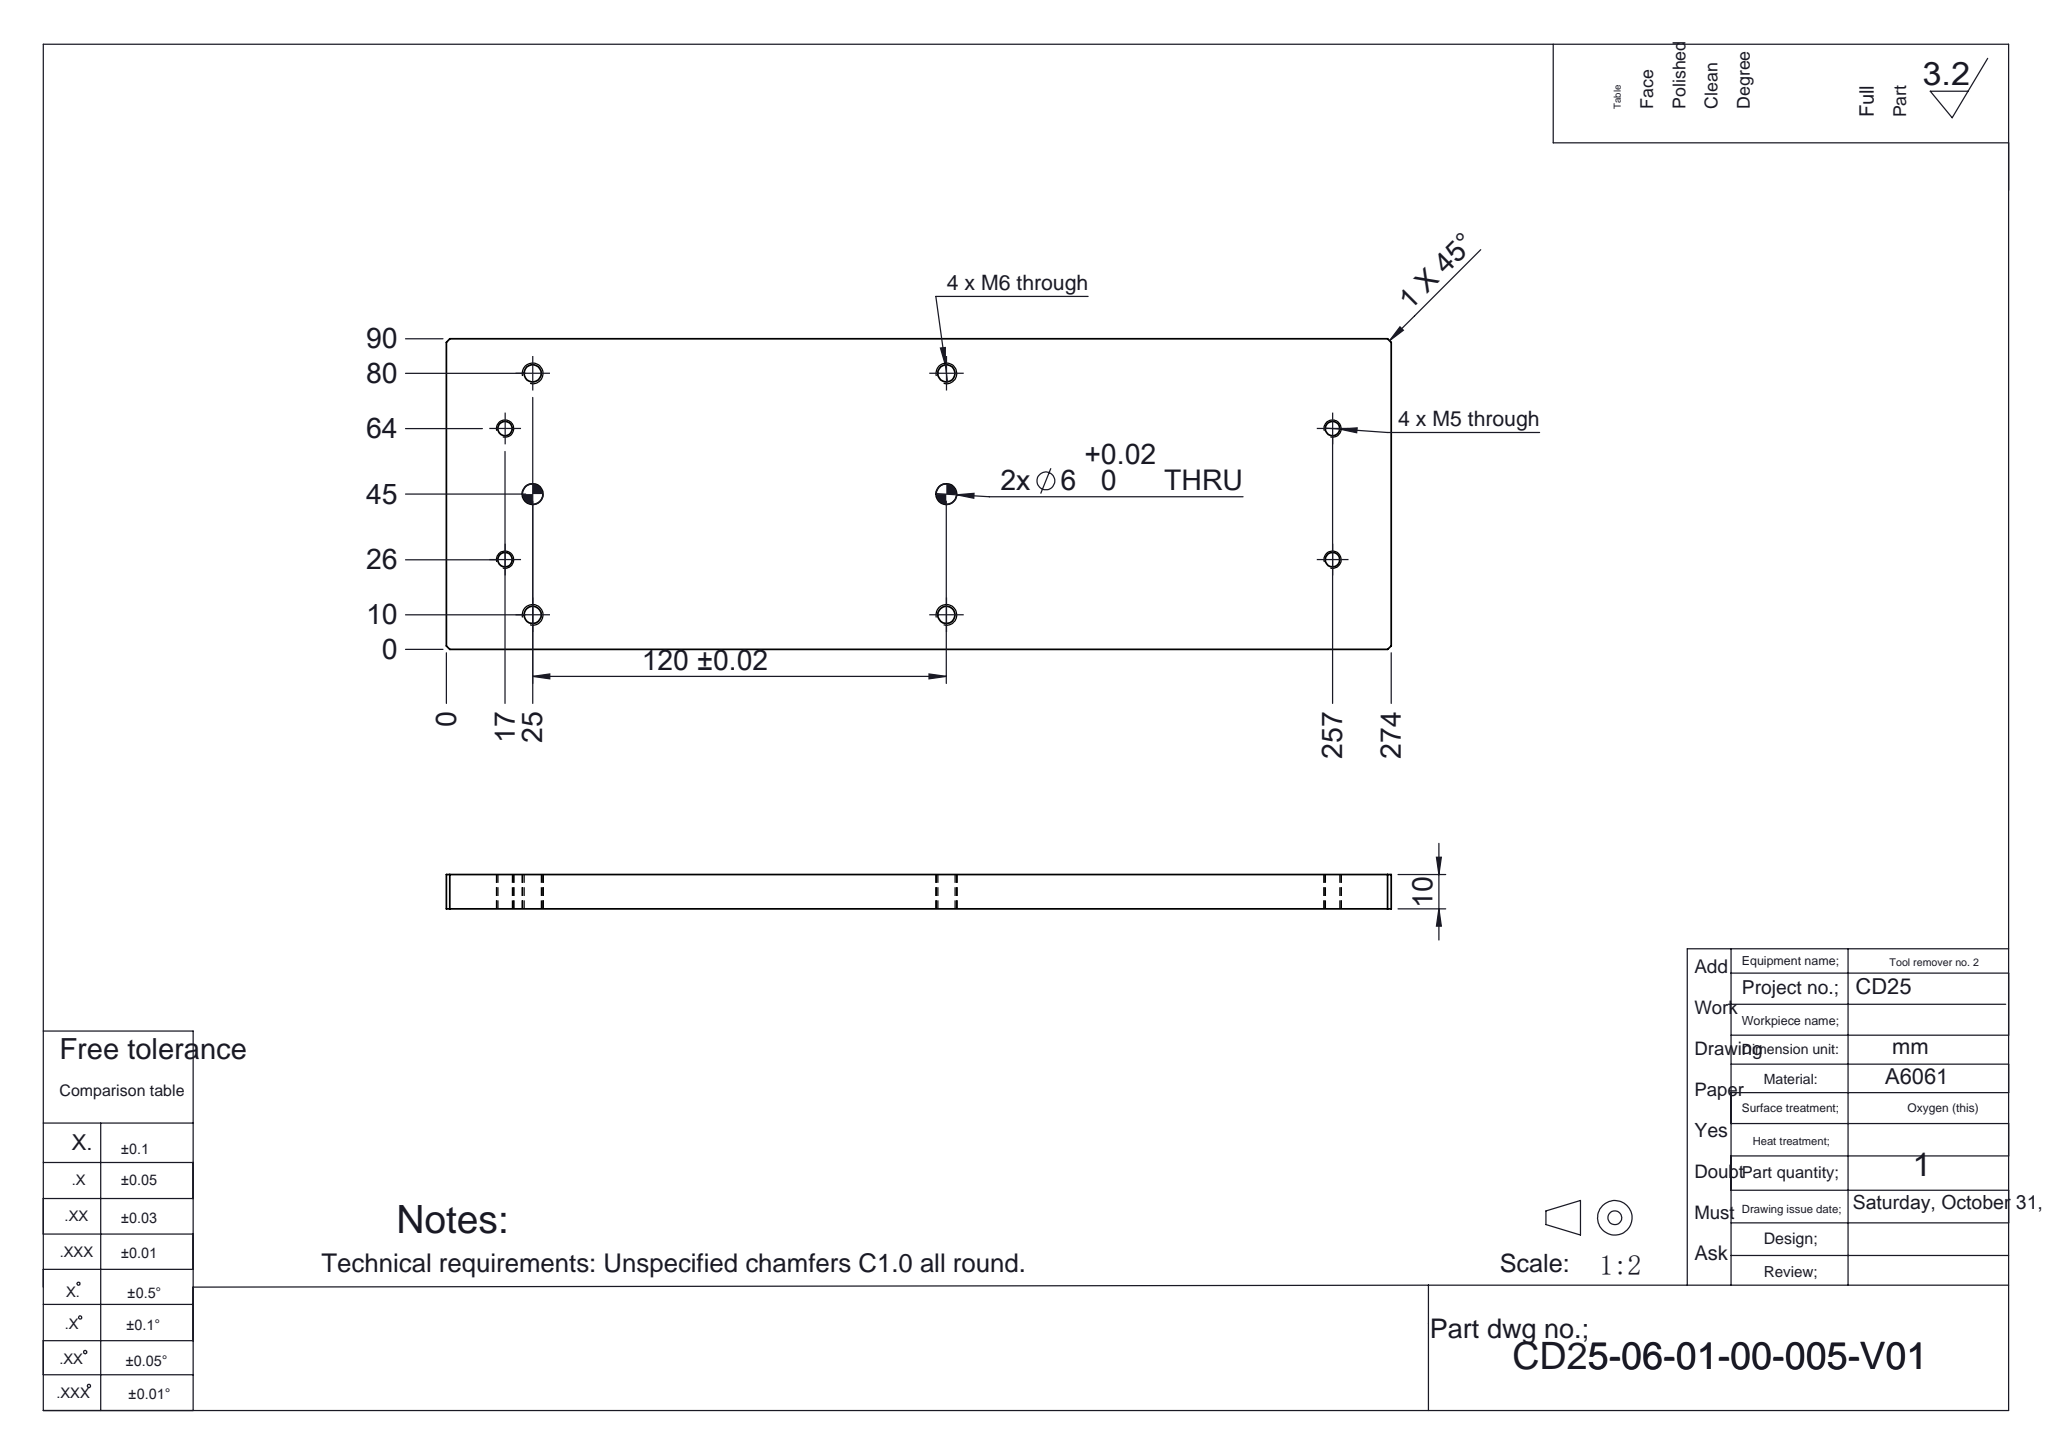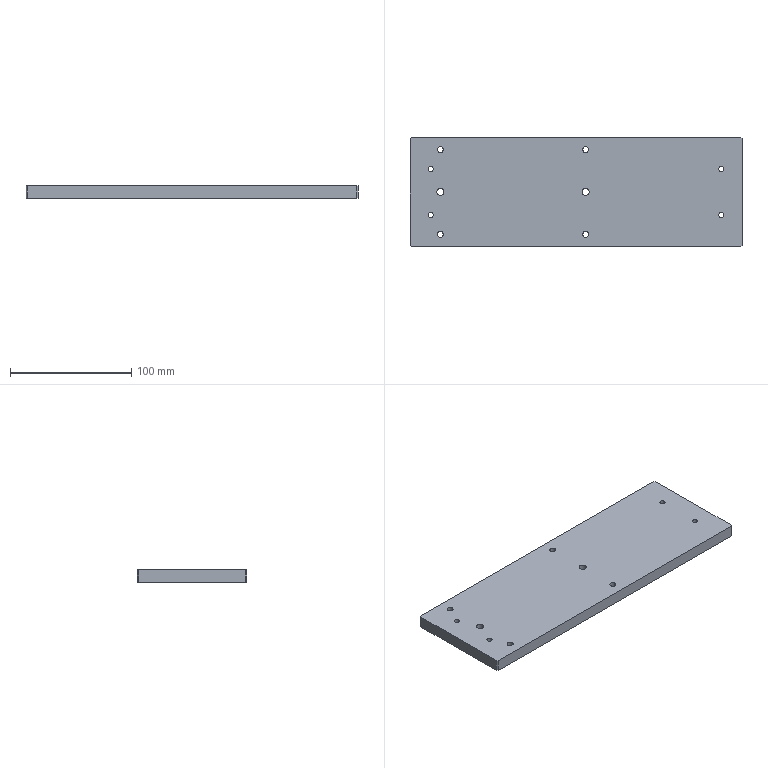Part | SolidWorks | features HoleWzd 3, Chamfer 1, Extrusion 1 | 1 solid | 30 faces | box 274 x 90 x 10 mm | volume 244675 mm3 | cylinder 20 | plane 10 | commonest cylinder face diameters 4.2 x8 5 x8 6 x4
STEP:
#1=CARTESIAN_POINT('',(-109.,0.,5.));
#2=VERTEX_POINT('',#1);
#3=CARTESIAN_POINT('',(-115.,0.,5.));
#4=VERTEX_POINT('',#3);
#5=CARTESIAN_POINT('',(-112.,0.,5.));
#6=DIRECTION('',(0.,0.,-1.));
#7=DIRECTION('',(-1.,0.,0.));
#8=AXIS2_PLACEMENT_3D('',#5,#6,#7);
#9=CIRCLE('',#8,3.);
#10=EDGE_CURVE('',#2,#4,#9,.T.);
#11=ORIENTED_EDGE('',*,*,#10,.F.);
#12=CARTESIAN_POINT('',(-109.,0.,-5.));
#13=VERTEX_POINT('',#12);
#14=CARTESIAN_POINT('',(-109.,0.,-5.));
#15=DIRECTION('',(0.,0.,-1.));
#16=VECTOR('',#15,1000.);
#17=LINE('',#14,#16);
#18=EDGE_CURVE('',#2,#13,#17,.T.);
#19=ORIENTED_EDGE('',*,*,#18,.T.);
#20=CARTESIAN_POINT('',(-115.,0.,-5.));
#21=VERTEX_POINT('',#20);
#22=CARTESIAN_POINT('',(-112.,0.,-5.));
#23=DIRECTION('',(0.,0.,-1.));
#24=DIRECTION('',(-1.,0.,0.));
#25=AXIS2_PLACEMENT_3D('',#22,#23,#24);
#26=CIRCLE('',#25,3.);
#27=EDGE_CURVE('',#13,#21,#26,.T.);
#28=ORIENTED_EDGE('',*,*,#27,.T.);
#29=CARTESIAN_POINT('',(-115.,0.,-5.));
#30=DIRECTION('',(0.,0.,-1.));
#31=VECTOR('',#30,1000.);
#32=LINE('',#29,#31);
#33=EDGE_CURVE('',#4,#21,#32,.T.);
#34=ORIENTED_EDGE('',*,*,#33,.F.);
#35=EDGE_LOOP('',(#11,#19,#28,#34));
#36=FACE_OUTER_BOUND('',#35,.T.);
#37=CARTESIAN_POINT('',(-112.,0.,-5.));
#38=DIRECTION('',(0.,0.,-1.));
#39=DIRECTION('',(-1.,0.,0.));
#40=AXIS2_PLACEMENT_3D('',#37,#38,#39);
#41=CYLINDRICAL_SURFACE('',#40,3.);
#42=ADVANCED_FACE('',(#36),#41,.F.);
#43=CARTESIAN_POINT('',(11.,0.,5.));
#44=VERTEX_POINT('',#43);
#45=CARTESIAN_POINT('',(5.,0.,5.));
#46=VERTEX_POINT('',#45);
#47=CARTESIAN_POINT('',(8.,0.,5.));
#48=DIRECTION('',(0.,0.,-1.));
#49=DIRECTION('',(-1.,0.,0.));
#50=AXIS2_PLACEMENT_3D('',#47,#48,#49);
#51=CIRCLE('',#50,3.);
#52=EDGE_CURVE('',#44,#46,#51,.T.);
#53=ORIENTED_EDGE('',*,*,#52,.F.);
#54=CARTESIAN_POINT('',(11.,0.,-5.));
#55=VERTEX_POINT('',#54);
#56=CARTESIAN_POINT('',(11.,0.,-5.));
#57=DIRECTION('',(0.,0.,-1.));
#58=VECTOR('',#57,1000.);
#59=LINE('',#56,#58);
#60=EDGE_CURVE('',#44,#55,#59,.T.);
#61=ORIENTED_EDGE('',*,*,#60,.T.);
#62=CARTESIAN_POINT('',(5.,0.,-5.));
#63=VERTEX_POINT('',#62);
#64=CARTESIAN_POINT('',(8.,0.,-5.));
#65=DIRECTION('',(0.,0.,-1.));
#66=DIRECTION('',(-1.,0.,0.));
#67=AXIS2_PLACEMENT_3D('',#64,#65,#66);
#68=CIRCLE('',#67,3.);
#69=EDGE_CURVE('',#55,#63,#68,.T.);
#70=ORIENTED_EDGE('',*,*,#69,.T.);
#71=CARTESIAN_POINT('',(5.,0.,-5.));
#72=DIRECTION('',(0.,0.,-1.));
#73=VECTOR('',#72,1000.);
#74=LINE('',#71,#73);
#75=EDGE_CURVE('',#46,#63,#74,.T.);
#76=ORIENTED_EDGE('',*,*,#75,.F.);
#77=EDGE_LOOP('',(#53,#61,#70,#76));
#78=FACE_OUTER_BOUND('',#77,.T.);
#79=CARTESIAN_POINT('',(8.,0.,-5.));
#80=DIRECTION('',(0.,0.,-1.));
#81=DIRECTION('',(-1.,0.,0.));
#82=AXIS2_PLACEMENT_3D('',#79,#80,#81);
#83=CYLINDRICAL_SURFACE('',#82,3.);
#84=ADVANCED_FACE('',(#78),#83,.F.);
#85=CARTESIAN_POINT('',(-109.5,35.,5.));
#86=VERTEX_POINT('',#85);
#87=CARTESIAN_POINT('',(-114.5,35.,5.));
#88=VERTEX_POINT('',#87);
#89=CARTESIAN_POINT('',(-112.,35.,5.));
#90=DIRECTION('',(0.,0.,-1.));
#91=DIRECTION('',(-1.,0.,0.));
#92=AXIS2_PLACEMENT_3D('',#89,#90,#91);
#93=CIRCLE('',#92,2.5);
#94=EDGE_CURVE('',#86,#88,#93,.T.);
#95=ORIENTED_EDGE('',*,*,#94,.F.);
#96=CARTESIAN_POINT('',(-109.5,35.,-5.));
#97=VERTEX_POINT('',#96);
#98=CARTESIAN_POINT('',(-109.5,35.,-5.));
#99=DIRECTION('',(0.,0.,-1.));
#100=VECTOR('',#99,1000.);
#101=LINE('',#98,#100);
#102=EDGE_CURVE('',#86,#97,#101,.T.);
#103=ORIENTED_EDGE('',*,*,#102,.T.);
#104=CARTESIAN_POINT('',(-114.5,35.,-5.));
#105=VERTEX_POINT('',#104);
#106=CARTESIAN_POINT('',(-112.,35.,-5.));
#107=DIRECTION('',(0.,0.,-1.));
#108=DIRECTION('',(-1.,0.,0.));
#109=AXIS2_PLACEMENT_3D('',#106,#107,#108);
#110=CIRCLE('',#109,2.5);
#111=EDGE_CURVE('',#97,#105,#110,.T.);
#112=ORIENTED_EDGE('',*,*,#111,.T.);
#113=CARTESIAN_POINT('',(-114.5,35.,-5.));
#114=DIRECTION('',(0.,0.,-1.));
#115=VECTOR('',#114,1000.);
#116=LINE('',#113,#115);
#117=EDGE_CURVE('',#88,#105,#116,.T.);
#118=ORIENTED_EDGE('',*,*,#117,.F.);
#119=EDGE_LOOP('',(#95,#103,#112,#118));
#120=FACE_OUTER_BOUND('',#119,.T.);
#121=CARTESIAN_POINT('',(-112.,35.,-5.));
#122=DIRECTION('',(0.,0.,-1.));
#123=DIRECTION('',(-1.,0.,0.));
#124=AXIS2_PLACEMENT_3D('',#121,#122,#123);
#125=CYLINDRICAL_SURFACE('',#124,2.5);
#126=ADVANCED_FACE('',(#120),#125,.F.);
#127=CARTESIAN_POINT('',(-109.5,-35.,5.));
#128=VERTEX_POINT('',#127);
#129=CARTESIAN_POINT('',(-114.5,-35.,5.));
#130=VERTEX_POINT('',#129);
#131=CARTESIAN_POINT('',(-112.,-35.,5.));
#132=DIRECTION('',(0.,0.,-1.));
#133=DIRECTION('',(-1.,0.,0.));
#134=AXIS2_PLACEMENT_3D('',#131,#132,#133);
#135=CIRCLE('',#134,2.5);
#136=EDGE_CURVE('',#128,#130,#135,.T.);
#137=ORIENTED_EDGE('',*,*,#136,.F.);
#138=CARTESIAN_POINT('',(-109.5,-35.,-5.));
#139=VERTEX_POINT('',#138);
#140=CARTESIAN_POINT('',(-109.5,-35.,-5.));
#141=DIRECTION('',(0.,0.,-1.));
#142=VECTOR('',#141,1000.);
#143=LINE('',#140,#142);
#144=EDGE_CURVE('',#128,#139,#143,.T.);
#145=ORIENTED_EDGE('',*,*,#144,.T.);
#146=CARTESIAN_POINT('',(-114.5,-35.,-5.));
#147=VERTEX_POINT('',#146);
#148=CARTESIAN_POINT('',(-112.,-35.,-5.));
#149=DIRECTION('',(0.,0.,-1.));
#150=DIRECTION('',(-1.,0.,0.));
#151=AXIS2_PLACEMENT_3D('',#148,#149,#150);
#152=CIRCLE('',#151,2.5);
#153=EDGE_CURVE('',#139,#147,#152,.T.);
#154=ORIENTED_EDGE('',*,*,#153,.T.);
#155=CARTESIAN_POINT('',(-114.5,-35.,-5.));
#156=DIRECTION('',(0.,0.,-1.));
#157=VECTOR('',#156,1000.);
#158=LINE('',#155,#157);
#159=EDGE_CURVE('',#130,#147,#158,.T.);
#160=ORIENTED_EDGE('',*,*,#159,.F.);
#161=EDGE_LOOP('',(#137,#145,#154,#160));
#162=FACE_OUTER_BOUND('',#161,.T.);
#163=CARTESIAN_POINT('',(-112.,-35.,-5.));
#164=DIRECTION('',(0.,0.,-1.));
#165=DIRECTION('',(-1.,0.,0.));
#166=AXIS2_PLACEMENT_3D('',#163,#164,#165);
#167=CYLINDRICAL_SURFACE('',#166,2.5);
#168=ADVANCED_FACE('',(#162),#167,.F.);
#169=CARTESIAN_POINT('',(10.5,-35.,5.));
#170=VERTEX_POINT('',#169);
#171=CARTESIAN_POINT('',(5.5,-35.,5.));
#172=VERTEX_POINT('',#171);
#173=CARTESIAN_POINT('',(8.,-35.,5.));
#174=DIRECTION('',(0.,0.,-1.));
#175=DIRECTION('',(-1.,0.,0.));
#176=AXIS2_PLACEMENT_3D('',#173,#174,#175);
#177=CIRCLE('',#176,2.5);
#178=EDGE_CURVE('',#170,#172,#177,.T.);
#179=ORIENTED_EDGE('',*,*,#178,.F.);
#180=CARTESIAN_POINT('',(10.5,-35.,-5.));
#181=VERTEX_POINT('',#180);
#182=CARTESIAN_POINT('',(10.5,-35.,-5.));
#183=DIRECTION('',(0.,0.,-1.));
#184=VECTOR('',#183,1000.);
#185=LINE('',#182,#184);
#186=EDGE_CURVE('',#170,#181,#185,.T.);
#187=ORIENTED_EDGE('',*,*,#186,.T.);
#188=CARTESIAN_POINT('',(5.5,-35.,-5.));
#189=VERTEX_POINT('',#188);
#190=CARTESIAN_POINT('',(8.,-35.,-5.));
#191=DIRECTION('',(0.,0.,-1.));
#192=DIRECTION('',(-1.,0.,0.));
#193=AXIS2_PLACEMENT_3D('',#190,#191,#192);
#194=CIRCLE('',#193,2.5);
#195=EDGE_CURVE('',#181,#189,#194,.T.);
#196=ORIENTED_EDGE('',*,*,#195,.T.);
#197=CARTESIAN_POINT('',(5.5,-35.,-5.));
#198=DIRECTION('',(0.,0.,-1.));
#199=VECTOR('',#198,1000.);
#200=LINE('',#197,#199);
#201=EDGE_CURVE('',#172,#189,#200,.T.);
#202=ORIENTED_EDGE('',*,*,#201,.F.);
#203=EDGE_LOOP('',(#179,#187,#196,#202));
#204=FACE_OUTER_BOUND('',#203,.T.);
#205=CARTESIAN_POINT('',(8.,-35.,-5.));
#206=DIRECTION('',(0.,0.,-1.));
#207=DIRECTION('',(-1.,0.,0.));
#208=AXIS2_PLACEMENT_3D('',#205,#206,#207);
#209=CYLINDRICAL_SURFACE('',#208,2.5);
#210=ADVANCED_FACE('',(#204),#209,.F.);
#211=CARTESIAN_POINT('',(10.5,35.,5.));
#212=VERTEX_POINT('',#211);
#213=CARTESIAN_POINT('',(5.5,35.,5.));
#214=VERTEX_POINT('',#213);
#215=CARTESIAN_POINT('',(8.,35.,5.));
#216=DIRECTION('',(0.,0.,-1.));
#217=DIRECTION('',(-1.,0.,0.));
#218=AXIS2_PLACEMENT_3D('',#215,#216,#217);
#219=CIRCLE('',#218,2.5);
#220=EDGE_CURVE('',#212,#214,#219,.T.);
#221=ORIENTED_EDGE('',*,*,#220,.F.);
#222=CARTESIAN_POINT('',(10.5,35.,-5.));
#223=VERTEX_POINT('',#222);
#224=CARTESIAN_POINT('',(10.5,35.,-5.));
#225=DIRECTION('',(0.,0.,-1.));
#226=VECTOR('',#225,1000.);
#227=LINE('',#224,#226);
#228=EDGE_CURVE('',#212,#223,#227,.T.);
#229=ORIENTED_EDGE('',*,*,#228,.T.);
#230=CARTESIAN_POINT('',(5.5,35.,-5.));
#231=VERTEX_POINT('',#230);
#232=CARTESIAN_POINT('',(8.,35.,-5.));
#233=DIRECTION('',(0.,0.,-1.));
#234=DIRECTION('',(-1.,0.,0.));
#235=AXIS2_PLACEMENT_3D('',#232,#233,#234);
#236=CIRCLE('',#235,2.5);
#237=EDGE_CURVE('',#223,#231,#236,.T.);
#238=ORIENTED_EDGE('',*,*,#237,.T.);
#239=CARTESIAN_POINT('',(5.5,35.,-5.));
#240=DIRECTION('',(0.,0.,-1.));
#241=VECTOR('',#240,1000.);
#242=LINE('',#239,#241);
#243=EDGE_CURVE('',#214,#231,#242,.T.);
#244=ORIENTED_EDGE('',*,*,#243,.F.);
#245=EDGE_LOOP('',(#221,#229,#238,#244));
#246=FACE_OUTER_BOUND('',#245,.T.);
#247=CARTESIAN_POINT('',(8.,35.,-5.));
#248=DIRECTION('',(0.,0.,-1.));
#249=DIRECTION('',(-1.,0.,0.));
#250=AXIS2_PLACEMENT_3D('',#247,#248,#249);
#251=CYLINDRICAL_SURFACE('',#250,2.5);
#252=ADVANCED_FACE('',(#246),#251,.F.);
#253=CARTESIAN_POINT('',(-122.1,19.,-5.));
#254=VERTEX_POINT('',#253);
#255=CARTESIAN_POINT('',(-117.9,19.,-5.));
#256=VERTEX_POINT('',#255);
#257=CARTESIAN_POINT('',(-120.,19.,-5.));
#258=DIRECTION('',(0.,0.,1.));
#259=DIRECTION('',(1.,0.,0.));
#260=AXIS2_PLACEMENT_3D('',#257,#258,#259);
#261=CIRCLE('',#260,2.1);
#262=EDGE_CURVE('',#254,#256,#261,.T.);
#263=ORIENTED_EDGE('',*,*,#262,.F.);
#264=CARTESIAN_POINT('',(-122.1,19.,5.));
#265=VERTEX_POINT('',#264);
#266=CARTESIAN_POINT('',(-122.1,19.,5.));
#267=DIRECTION('',(0.,0.,1.));
#268=VECTOR('',#267,1000.);
#269=LINE('',#266,#268);
#270=EDGE_CURVE('',#254,#265,#269,.T.);
#271=ORIENTED_EDGE('',*,*,#270,.T.);
#272=CARTESIAN_POINT('',(-117.9,19.,5.));
#273=VERTEX_POINT('',#272);
#274=CARTESIAN_POINT('',(-120.,19.,5.));
#275=DIRECTION('',(0.,0.,1.));
#276=DIRECTION('',(1.,0.,0.));
#277=AXIS2_PLACEMENT_3D('',#274,#275,#276);
#278=CIRCLE('',#277,2.1);
#279=EDGE_CURVE('',#265,#273,#278,.T.);
#280=ORIENTED_EDGE('',*,*,#279,.T.);
#281=CARTESIAN_POINT('',(-117.9,19.,5.));
#282=DIRECTION('',(0.,0.,1.));
#283=VECTOR('',#282,1000.);
#284=LINE('',#281,#283);
#285=EDGE_CURVE('',#256,#273,#284,.T.);
#286=ORIENTED_EDGE('',*,*,#285,.F.);
#287=EDGE_LOOP('',(#263,#271,#280,#286));
#288=FACE_OUTER_BOUND('',#287,.T.);
#289=CARTESIAN_POINT('',(-120.,19.,5.));
#290=DIRECTION('',(0.,0.,1.));
#291=DIRECTION('',(1.,0.,0.));
#292=AXIS2_PLACEMENT_3D('',#289,#290,#291);
#293=CYLINDRICAL_SURFACE('',#292,2.1);
#294=ADVANCED_FACE('',(#288),#293,.F.);
#295=CARTESIAN_POINT('',(-122.1,-19.,-5.));
#296=VERTEX_POINT('',#295);
#297=CARTESIAN_POINT('',(-117.9,-19.,-5.));
#298=VERTEX_POINT('',#297);
#299=CARTESIAN_POINT('',(-120.,-19.,-5.));
#300=DIRECTION('',(0.,0.,1.));
#301=DIRECTION('',(1.,0.,0.));
#302=AXIS2_PLACEMENT_3D('',#299,#300,#301);
#303=CIRCLE('',#302,2.1);
#304=EDGE_CURVE('',#296,#298,#303,.T.);
#305=ORIENTED_EDGE('',*,*,#304,.F.);
#306=CARTESIAN_POINT('',(-122.1,-19.,5.));
#307=VERTEX_POINT('',#306);
#308=CARTESIAN_POINT('',(-122.1,-19.,5.));
#309=DIRECTION('',(0.,0.,1.));
#310=VECTOR('',#309,1000.);
#311=LINE('',#308,#310);
#312=EDGE_CURVE('',#296,#307,#311,.T.);
#313=ORIENTED_EDGE('',*,*,#312,.T.);
#314=CARTESIAN_POINT('',(-117.9,-19.,5.));
#315=VERTEX_POINT('',#314);
#316=CARTESIAN_POINT('',(-120.,-19.,5.));
#317=DIRECTION('',(0.,0.,1.));
#318=DIRECTION('',(1.,0.,0.));
#319=AXIS2_PLACEMENT_3D('',#316,#317,#318);
#320=CIRCLE('',#319,2.1);
#321=EDGE_CURVE('',#307,#315,#320,.T.);
#322=ORIENTED_EDGE('',*,*,#321,.T.);
#323=CARTESIAN_POINT('',(-117.9,-19.,5.));
#324=DIRECTION('',(0.,0.,1.));
#325=VECTOR('',#324,1000.);
#326=LINE('',#323,#325);
#327=EDGE_CURVE('',#298,#315,#326,.T.);
#328=ORIENTED_EDGE('',*,*,#327,.F.);
#329=EDGE_LOOP('',(#305,#313,#322,#328));
#330=FACE_OUTER_BOUND('',#329,.T.);
#331=CARTESIAN_POINT('',(-120.,-19.,5.));
#332=DIRECTION('',(0.,0.,1.));
#333=DIRECTION('',(1.,0.,0.));
#334=AXIS2_PLACEMENT_3D('',#331,#332,#333);
#335=CYLINDRICAL_SURFACE('',#334,2.1);
#336=ADVANCED_FACE('',(#330),#335,.F.);
#337=CARTESIAN_POINT('',(117.9,-19.,-5.));
#338=VERTEX_POINT('',#337);
#339=CARTESIAN_POINT('',(122.1,-19.,-5.));
#340=VERTEX_POINT('',#339);
#341=CARTESIAN_POINT('',(120.,-19.,-5.));
#342=DIRECTION('',(0.,0.,1.));
#343=DIRECTION('',(1.,0.,0.));
#344=AXIS2_PLACEMENT_3D('',#341,#342,#343);
#345=CIRCLE('',#344,2.1);
#346=EDGE_CURVE('',#338,#340,#345,.T.);
#347=ORIENTED_EDGE('',*,*,#346,.F.);
#348=CARTESIAN_POINT('',(117.9,-19.,5.));
#349=VERTEX_POINT('',#348);
#350=CARTESIAN_POINT('',(117.9,-19.,5.));
#351=DIRECTION('',(0.,0.,1.));
#352=VECTOR('',#351,1000.);
#353=LINE('',#350,#352);
#354=EDGE_CURVE('',#338,#349,#353,.T.);
#355=ORIENTED_EDGE('',*,*,#354,.T.);
#356=CARTESIAN_POINT('',(122.1,-19.,5.));
#357=VERTEX_POINT('',#356);
#358=CARTESIAN_POINT('',(120.,-19.,5.));
#359=DIRECTION('',(0.,0.,1.));
#360=DIRECTION('',(1.,0.,0.));
#361=AXIS2_PLACEMENT_3D('',#358,#359,#360);
#362=CIRCLE('',#361,2.1);
#363=EDGE_CURVE('',#349,#357,#362,.T.);
#364=ORIENTED_EDGE('',*,*,#363,.T.);
#365=CARTESIAN_POINT('',(122.1,-19.,5.));
#366=DIRECTION('',(0.,0.,1.));
#367=VECTOR('',#366,1000.);
#368=LINE('',#365,#367);
#369=EDGE_CURVE('',#340,#357,#368,.T.);
#370=ORIENTED_EDGE('',*,*,#369,.F.);
#371=EDGE_LOOP('',(#347,#355,#364,#370));
#372=FACE_OUTER_BOUND('',#371,.T.);
#373=CARTESIAN_POINT('',(120.,-19.,5.));
#374=DIRECTION('',(0.,0.,1.));
#375=DIRECTION('',(1.,0.,0.));
#376=AXIS2_PLACEMENT_3D('',#373,#374,#375);
#377=CYLINDRICAL_SURFACE('',#376,2.1);
#378=ADVANCED_FACE('',(#372),#377,.F.);
#379=CARTESIAN_POINT('',(117.9,19.,-5.));
#380=VERTEX_POINT('',#379);
#381=CARTESIAN_POINT('',(122.1,19.,-5.));
#382=VERTEX_POINT('',#381);
#383=CARTESIAN_POINT('',(120.,19.,-5.));
#384=DIRECTION('',(0.,0.,1.));
#385=DIRECTION('',(1.,0.,0.));
#386=AXIS2_PLACEMENT_3D('',#383,#384,#385);
#387=CIRCLE('',#386,2.1);
#388=EDGE_CURVE('',#380,#382,#387,.T.);
#389=ORIENTED_EDGE('',*,*,#388,.F.);
#390=CARTESIAN_POINT('',(117.9,19.,5.));
#391=VERTEX_POINT('',#390);
#392=CARTESIAN_POINT('',(117.9,19.,5.));
#393=DIRECTION('',(0.,0.,1.));
#394=VECTOR('',#393,1000.);
#395=LINE('',#392,#394);
#396=EDGE_CURVE('',#380,#391,#395,.T.);
#397=ORIENTED_EDGE('',*,*,#396,.T.);
#398=CARTESIAN_POINT('',(122.1,19.,5.));
#399=VERTEX_POINT('',#398);
#400=CARTESIAN_POINT('',(120.,19.,5.));
#401=DIRECTION('',(0.,0.,1.));
#402=DIRECTION('',(1.,0.,0.));
#403=AXIS2_PLACEMENT_3D('',#400,#401,#402);
#404=CIRCLE('',#403,2.1);
#405=EDGE_CURVE('',#391,#399,#404,.T.);
#406=ORIENTED_EDGE('',*,*,#405,.T.);
#407=CARTESIAN_POINT('',(122.1,19.,5.));
#408=DIRECTION('',(0.,0.,1.));
#409=VECTOR('',#408,1000.);
#410=LINE('',#407,#409);
#411=EDGE_CURVE('',#382,#399,#410,.T.);
#412=ORIENTED_EDGE('',*,*,#411,.F.);
#413=EDGE_LOOP('',(#389,#397,#406,#412));
#414=FACE_OUTER_BOUND('',#413,.T.);
#415=CARTESIAN_POINT('',(120.,19.,5.));
#416=DIRECTION('',(0.,0.,1.));
#417=DIRECTION('',(1.,0.,0.));
#418=AXIS2_PLACEMENT_3D('',#415,#416,#417);
#419=CYLINDRICAL_SURFACE('',#418,2.1);
#420=ADVANCED_FACE('',(#414),#419,.F.);
#421=CARTESIAN_POINT('',(-112.,0.,5.));
#422=DIRECTION('',(0.,0.,-1.));
#423=DIRECTION('',(-1.,0.,0.));
#424=AXIS2_PLACEMENT_3D('',#421,#422,#423);
#425=CIRCLE('',#424,3.);
#426=EDGE_CURVE('',#4,#2,#425,.T.);
#427=ORIENTED_EDGE('',*,*,#426,.T.);
#428=ORIENTED_EDGE('',*,*,#10,.T.);
#429=EDGE_LOOP('',(#427,#428));
#430=FACE_BOUND('',#429,.T.);
#431=CARTESIAN_POINT('',(8.,0.,5.));
#432=DIRECTION('',(0.,0.,-1.));
#433=DIRECTION('',(-1.,0.,0.));
#434=AXIS2_PLACEMENT_3D('',#431,#432,#433);
#435=CIRCLE('',#434,3.);
#436=EDGE_CURVE('',#46,#44,#435,.T.);
#437=ORIENTED_EDGE('',*,*,#436,.T.);
#438=ORIENTED_EDGE('',*,*,#52,.T.);
#439=EDGE_LOOP('',(#437,#438));
#440=FACE_BOUND('',#439,.T.);
#441=CARTESIAN_POINT('',(-112.,35.,5.));
#442=DIRECTION('',(0.,0.,-1.));
#443=DIRECTION('',(-1.,0.,0.));
#444=AXIS2_PLACEMENT_3D('',#441,#442,#443);
#445=CIRCLE('',#444,2.5);
#446=EDGE_CURVE('',#88,#86,#445,.T.);
#447=ORIENTED_EDGE('',*,*,#446,.T.);
#448=ORIENTED_EDGE('',*,*,#94,.T.);
#449=EDGE_LOOP('',(#447,#448));
#450=FACE_BOUND('',#449,.T.);
#451=CARTESIAN_POINT('',(-112.,-35.,5.));
#452=DIRECTION('',(0.,0.,-1.));
#453=DIRECTION('',(-1.,0.,0.));
#454=AXIS2_PLACEMENT_3D('',#451,#452,#453);
#455=CIRCLE('',#454,2.5);
#456=EDGE_CURVE('',#130,#128,#455,.T.);
#457=ORIENTED_EDGE('',*,*,#456,.T.);
#458=ORIENTED_EDGE('',*,*,#136,.T.);
#459=EDGE_LOOP('',(#457,#458));
#460=FACE_BOUND('',#459,.T.);
#461=CARTESIAN_POINT('',(-136.,-45.,5.));
#462=VERTEX_POINT('',#461);
#463=CARTESIAN_POINT('',(136.,-45.,5.));
#464=VERTEX_POINT('',#463);
#465=CARTESIAN_POINT('',(-137.,-45.,5.));
#466=DIRECTION('',(1.,0.,0.));
#467=VECTOR('',#466,1000.);
#468=LINE('',#465,#467);
#469=EDGE_CURVE('',#462,#464,#468,.T.);
#470=ORIENTED_EDGE('',*,*,#469,.T.);
#471=CARTESIAN_POINT('',(137.,-44.,5.));
#472=VERTEX_POINT('',#471);
#473=CARTESIAN_POINT('',(90.5,-90.5,5.));
#474=DIRECTION('',(0.7071,0.7071,0.));
#475=VECTOR('',#474,1000.);
#476=LINE('',#473,#475);
#477=EDGE_CURVE('',#464,#472,#476,.T.);
#478=ORIENTED_EDGE('',*,*,#477,.T.);
#479=CARTESIAN_POINT('',(137.,44.,5.));
#480=VERTEX_POINT('',#479);
#481=CARTESIAN_POINT('',(137.,45.,5.));
#482=DIRECTION('',(0.,1.,0.));
#483=VECTOR('',#482,1000.);
#484=LINE('',#481,#483);
#485=EDGE_CURVE('',#472,#480,#484,.T.);
#486=ORIENTED_EDGE('',*,*,#485,.T.);
#487=CARTESIAN_POINT('',(136.,45.,5.));
#488=VERTEX_POINT('',#487);
#489=CARTESIAN_POINT('',(90.5,90.5,5.));
#490=DIRECTION('',(-0.7071,0.7071,0.));
#491=VECTOR('',#490,1000.);
#492=LINE('',#489,#491);
#493=EDGE_CURVE('',#480,#488,#492,.T.);
#494=ORIENTED_EDGE('',*,*,#493,.T.);
#495=CARTESIAN_POINT('',(-136.,45.,5.));
#496=VERTEX_POINT('',#495);
#497=CARTESIAN_POINT('',(-137.,45.,5.));
#498=DIRECTION('',(-1.,0.,0.));
#499=VECTOR('',#498,1000.);
#500=LINE('',#497,#499);
#501=EDGE_CURVE('',#488,#496,#500,.T.);
#502=ORIENTED_EDGE('',*,*,#501,.T.);
#503=CARTESIAN_POINT('',(-137.,44.,5.));
#504=VERTEX_POINT('',#503);
#505=CARTESIAN_POINT('',(-90.5,90.5,5.));
#506=DIRECTION('',(-0.7071,-0.7071,0.));
#507=VECTOR('',#506,1000.);
#508=LINE('',#505,#507);
#509=EDGE_CURVE('',#496,#504,#508,.T.);
#510=ORIENTED_EDGE('',*,*,#509,.T.);
#511=CARTESIAN_POINT('',(-137.,-44.,5.));
#512=VERTEX_POINT('',#511);
#513=CARTESIAN_POINT('',(-137.,45.,5.));
#514=DIRECTION('',(0.,-1.,0.));
#515=VECTOR('',#514,1000.);
#516=LINE('',#513,#515);
#517=EDGE_CURVE('',#504,#512,#516,.T.);
#518=ORIENTED_EDGE('',*,*,#517,.T.);
#519=CARTESIAN_POINT('',(-90.5,-90.5,5.));
#520=DIRECTION('',(0.7071,-0.7071,0.));
#521=VECTOR('',#520,1000.);
#522=LINE('',#519,#521);
#523=EDGE_CURVE('',#512,#462,#522,.T.);
#524=ORIENTED_EDGE('',*,*,#523,.T.);
#525=EDGE_LOOP('',(#470,#478,#486,#494,#502,#510,#518,#524));
#526=FACE_OUTER_BOUND('',#525,.T.);
#527=CARTESIAN_POINT('',(120.,19.,5.));
#528=DIRECTION('',(0.,0.,1.));
#529=DIRECTION('',(1.,0.,0.));
#530=AXIS2_PLACEMENT_3D('',#527,#528,#529);
#531=CIRCLE('',#530,2.1);
#532=EDGE_CURVE('',#399,#391,#531,.T.);
#533=ORIENTED_EDGE('',*,*,#532,.F.);
#534=ORIENTED_EDGE('',*,*,#405,.F.);
#535=EDGE_LOOP('',(#533,#534));
#536=FACE_BOUND('',#535,.T.);
#537=CARTESIAN_POINT('',(120.,-19.,5.));
#538=DIRECTION('',(0.,0.,1.));
#539=DIRECTION('',(1.,0.,0.));
#540=AXIS2_PLACEMENT_3D('',#537,#538,#539);
#541=CIRCLE('',#540,2.1);
#542=EDGE_CURVE('',#357,#349,#541,.T.);
#543=ORIENTED_EDGE('',*,*,#542,.F.);
#544=ORIENTED_EDGE('',*,*,#363,.F.);
#545=EDGE_LOOP('',(#543,#544));
#546=FACE_BOUND('',#545,.T.);
#547=CARTESIAN_POINT('',(-120.,-19.,5.));
#548=DIRECTION('',(0.,0.,1.));
#549=DIRECTION('',(1.,0.,0.));
#550=AXIS2_PLACEMENT_3D('',#547,#548,#549);
#551=CIRCLE('',#550,2.1);
#552=EDGE_CURVE('',#315,#307,#551,.T.);
#553=ORIENTED_EDGE('',*,*,#552,.F.);
#554=ORIENTED_EDGE('',*,*,#321,.F.);
#555=EDGE_LOOP('',(#553,#554));
#556=FACE_BOUND('',#555,.T.);
#557=CARTESIAN_POINT('',(-120.,19.,5.));
#558=DIRECTION('',(0.,0.,1.));
#559=DIRECTION('',(1.,0.,0.));
#560=AXIS2_PLACEMENT_3D('',#557,#558,#559);
#561=CIRCLE('',#560,2.1);
#562=EDGE_CURVE('',#273,#265,#561,.T.);
#563=ORIENTED_EDGE('',*,*,#562,.F.);
#564=ORIENTED_EDGE('',*,*,#279,.F.);
#565=EDGE_LOOP('',(#563,#564));
#566=FACE_BOUND('',#565,.T.);
#567=CARTESIAN_POINT('',(8.,35.,5.));
#568=DIRECTION('',(0.,0.,-1.));
#569=DIRECTION('',(-1.,0.,0.));
#570=AXIS2_PLACEMENT_3D('',#567,#568,#569);
#571=CIRCLE('',#570,2.5);
#572=EDGE_CURVE('',#214,#212,#571,.T.);
#573=ORIENTED_EDGE('',*,*,#572,.T.);
#574=ORIENTED_EDGE('',*,*,#220,.T.);
#575=EDGE_LOOP('',(#573,#574));
#576=FACE_BOUND('',#575,.T.);
#577=CARTESIAN_POINT('',(8.,-35.,5.));
#578=DIRECTION('',(0.,0.,-1.));
#579=DIRECTION('',(-1.,0.,0.));
#580=AXIS2_PLACEMENT_3D('',#577,#578,#579);
#581=CIRCLE('',#580,2.5);
#582=EDGE_CURVE('',#172,#170,#581,.T.);
#583=ORIENTED_EDGE('',*,*,#582,.T.);
#584=ORIENTED_EDGE('',*,*,#178,.T.);
#585=EDGE_LOOP('',(#583,#584));
#586=FACE_BOUND('',#585,.T.);
#587=CARTESIAN_POINT('',(0.,0.,5.));
#588=DIRECTION('',(0.,0.,1.));
#589=DIRECTION('',(1.,0.,0.));
#590=AXIS2_PLACEMENT_3D('',#587,#588,#589);
#591=PLANE('',#590);
#592=ADVANCED_FACE('',(#430,#440,#450,#460,#526,#536,#546,#556,#566,#576,#586),#591,.T.);
#593=ORIENTED_EDGE('',*,*,#485,.F.);
#594=CARTESIAN_POINT('',(137.,-44.,-5.));
#595=VERTEX_POINT('',#594);
#596=CARTESIAN_POINT('',(137.,-44.,5.));
#597=DIRECTION('',(0.,0.,-1.));
#598=VECTOR('',#597,1000.);
#599=LINE('',#596,#598);
#600=EDGE_CURVE('',#472,#595,#599,.T.);
#601=ORIENTED_EDGE('',*,*,#600,.T.);
#602=CARTESIAN_POINT('',(137.,44.,-5.));
#603=VERTEX_POINT('',#602);
#604=CARTESIAN_POINT('',(137.,45.,-5.));
#605=DIRECTION('',(0.,1.,0.));
#606=VECTOR('',#605,1000.);
#607=LINE('',#604,#606);
#608=EDGE_CURVE('',#595,#603,#607,.T.);
#609=ORIENTED_EDGE('',*,*,#608,.T.);
#610=CARTESIAN_POINT('',(137.,44.,5.));
#611=DIRECTION('',(0.,0.,1.));
#612=VECTOR('',#611,1000.);
#613=LINE('',#610,#612);
#614=EDGE_CURVE('',#603,#480,#613,.T.);
#615=ORIENTED_EDGE('',*,*,#614,.T.);
#616=EDGE_LOOP('',(#593,#601,#609,#615));
#617=FACE_OUTER_BOUND('',#616,.T.);
#618=CARTESIAN_POINT('',(137.,45.,5.));
#619=DIRECTION('',(-1.,0.,0.));
#620=DIRECTION('',(0.,-1.,0.));
#621=AXIS2_PLACEMENT_3D('',#618,#619,#620);
#622=PLANE('',#621);
#623=ADVANCED_FACE('',(#617),#622,.F.);
#624=CARTESIAN_POINT('',(136.,45.,-5.));
#625=VERTEX_POINT('',#624);
#626=CARTESIAN_POINT('',(-136.,45.,-5.));
#627=VERTEX_POINT('',#626);
#628=CARTESIAN_POINT('',(-137.,45.,-5.));
#629=DIRECTION('',(-1.,0.,0.));
#630=VECTOR('',#629,1000.);
#631=LINE('',#628,#630);
#632=EDGE_CURVE('',#625,#627,#631,.T.);
#633=ORIENTED_EDGE('',*,*,#632,.T.);
#634=CARTESIAN_POINT('',(-136.,45.,5.));
#635=DIRECTION('',(0.,0.,1.));
#636=VECTOR('',#635,1000.);
#637=LINE('',#634,#636);
#638=EDGE_CURVE('',#627,#496,#637,.T.);
#639=ORIENTED_EDGE('',*,*,#638,.T.);
#640=ORIENTED_EDGE('',*,*,#501,.F.);
#641=CARTESIAN_POINT('',(136.,45.,5.));
#642=DIRECTION('',(0.,0.,-1.));
#643=VECTOR('',#642,1000.);
#644=LINE('',#641,#643);
#645=EDGE_CURVE('',#488,#625,#644,.T.);
#646=ORIENTED_EDGE('',*,*,#645,.T.);
#647=EDGE_LOOP('',(#633,#639,#640,#646));
#648=FACE_OUTER_BOUND('',#647,.T.);
#649=CARTESIAN_POINT('',(-137.,45.,5.));
#650=DIRECTION('',(0.,-1.,0.));
#651=DIRECTION('',(0.,0.,-1.));
#652=AXIS2_PLACEMENT_3D('',#649,#650,#651);
#653=PLANE('',#652);
#654=ADVANCED_FACE('',(#648),#653,.F.);
#655=CARTESIAN_POINT('',(-137.,44.,-5.));
#656=VERTEX_POINT('',#655);
#657=CARTESIAN_POINT('',(-137.,-44.,-5.));
#658=VERTEX_POINT('',#657);
#659=CARTESIAN_POINT('',(-137.,45.,-5.));
#660=DIRECTION('',(0.,-1.,0.));
#661=VECTOR('',#660,1000.);
#662=LINE('',#659,#661);
#663=EDGE_CURVE('',#656,#658,#662,.T.);
#664=ORIENTED_EDGE('',*,*,#663,.T.);
#665=CARTESIAN_POINT('',(-137.,-44.,5.));
#666=DIRECTION('',(0.,0.,1.));
#667=VECTOR('',#666,1000.);
#668=LINE('',#665,#667);
#669=EDGE_CURVE('',#658,#512,#668,.T.);
#670=ORIENTED_EDGE('',*,*,#669,.T.);
#671=ORIENTED_EDGE('',*,*,#517,.F.);
#672=CARTESIAN_POINT('',(-137.,44.,5.));
#673=DIRECTION('',(0.,0.,-1.));
#674=VECTOR('',#673,1000.);
#675=LINE('',#672,#674);
#676=EDGE_CURVE('',#504,#656,#675,.T.);
#677=ORIENTED_EDGE('',*,*,#676,.T.);
#678=EDGE_LOOP('',(#664,#670,#671,#677));
#679=FACE_OUTER_BOUND('',#678,.T.);
#680=CARTESIAN_POINT('',(-137.,45.,5.));
#681=DIRECTION('',(1.,0.,0.));
#682=DIRECTION('',(0.,0.,-1.));
#683=AXIS2_PLACEMENT_3D('',#680,#681,#682);
#684=PLANE('',#683);
#685=ADVANCED_FACE('',(#679),#684,.F.);
#686=CARTESIAN_POINT('',(-136.,-45.,-5.));
#687=VERTEX_POINT('',#686);
#688=CARTESIAN_POINT('',(136.,-45.,-5.));
#689=VERTEX_POINT('',#688);
#690=CARTESIAN_POINT('',(-137.,-45.,-5.));
#691=DIRECTION('',(1.,0.,0.));
#692=VECTOR('',#691,1000.);
#693=LINE('',#690,#692);
#694=EDGE_CURVE('',#687,#689,#693,.T.);
#695=ORIENTED_EDGE('',*,*,#694,.T.);
#696=CARTESIAN_POINT('',(136.,-45.,5.));
#697=DIRECTION('',(0.,0.,1.));
#698=VECTOR('',#697,1000.);
#699=LINE('',#696,#698);
#700=EDGE_CURVE('',#689,#464,#699,.T.);
#701=ORIENTED_EDGE('',*,*,#700,.T.);
#702=ORIENTED_EDGE('',*,*,#469,.F.);
#703=CARTESIAN_POINT('',(-136.,-45.,5.));
#704=DIRECTION('',(0.,0.,-1.));
#705=VECTOR('',#704,1000.);
#706=LINE('',#703,#705);
#707=EDGE_CURVE('',#462,#687,#706,.T.);
#708=ORIENTED_EDGE('',*,*,#707,.T.);
#709=EDGE_LOOP('',(#695,#701,#702,#708));
#710=FACE_OUTER_BOUND('',#709,.T.);
#711=CARTESIAN_POINT('',(-137.,-45.,5.));
#712=DIRECTION('',(0.,1.,0.));
#713=DIRECTION('',(0.,0.,1.));
#714=AXIS2_PLACEMENT_3D('',#711,#712,#713);
#715=PLANE('',#714);
#716=ADVANCED_FACE('',(#710),#715,.F.);
#717=CARTESIAN_POINT('',(-112.,0.,-5.));
#718=DIRECTION('',(0.,0.,-1.));
#719=DIRECTION('',(-1.,0.,0.));
#720=AXIS2_PLACEMENT_3D('',#717,#718,#719);
#721=CIRCLE('',#720,3.);
#722=EDGE_CURVE('',#21,#13,#721,.T.);
#723=ORIENTED_EDGE('',*,*,#722,.F.);
#724=ORIENTED_EDGE('',*,*,#27,.F.);
#725=EDGE_LOOP('',(#723,#724));
#726=FACE_BOUND('',#725,.T.);
#727=CARTESIAN_POINT('',(8.,0.,-5.));
#728=DIRECTION('',(0.,0.,-1.));
#729=DIRECTION('',(-1.,0.,0.));
#730=AXIS2_PLACEMENT_3D('',#727,#728,#729);
#731=CIRCLE('',#730,3.);
#732=EDGE_CURVE('',#63,#55,#731,.T.);
#733=ORIENTED_EDGE('',*,*,#732,.F.);
#734=ORIENTED_EDGE('',*,*,#69,.F.);
#735=EDGE_LOOP('',(#733,#734));
#736=FACE_BOUND('',#735,.T.);
#737=CARTESIAN_POINT('',(-112.,35.,-5.));
#738=DIRECTION('',(0.,0.,-1.));
#739=DIRECTION('',(-1.,0.,0.));
#740=AXIS2_PLACEMENT_3D('',#737,#738,#739);
#741=CIRCLE('',#740,2.5);
#742=EDGE_CURVE('',#105,#97,#741,.T.);
#743=ORIENTED_EDGE('',*,*,#742,.F.);
#744=ORIENTED_EDGE('',*,*,#111,.F.);
#745=EDGE_LOOP('',(#743,#744));
#746=FACE_BOUND('',#745,.T.);
#747=CARTESIAN_POINT('',(-112.,-35.,-5.));
#748=DIRECTION('',(0.,0.,-1.));
#749=DIRECTION('',(-1.,0.,0.));
#750=AXIS2_PLACEMENT_3D('',#747,#748,#749);
#751=CIRCLE('',#750,2.5);
#752=EDGE_CURVE('',#147,#139,#751,.T.);
#753=ORIENTED_EDGE('',*,*,#752,.F.);
#754=ORIENTED_EDGE('',*,*,#153,.F.);
#755=EDGE_LOOP('',(#753,#754));
#756=FACE_BOUND('',#755,.T.);
#757=CARTESIAN_POINT('',(8.,-35.,-5.));
#758=DIRECTION('',(0.,0.,-1.));
#759=DIRECTION('',(-1.,0.,0.));
#760=AXIS2_PLACEMENT_3D('',#757,#758,#759);
#761=CIRCLE('',#760,2.5);
#762=EDGE_CURVE('',#189,#181,#761,.T.);
#763=ORIENTED_EDGE('',*,*,#762,.F.);
#764=ORIENTED_EDGE('',*,*,#195,.F.);
#765=EDGE_LOOP('',(#763,#764));
#766=FACE_BOUND('',#765,.T.);
#767=CARTESIAN_POINT('',(8.,35.,-5.));
#768=DIRECTION('',(0.,0.,-1.));
#769=DIRECTION('',(-1.,0.,0.));
#770=AXIS2_PLACEMENT_3D('',#767,#768,#769);
#771=CIRCLE('',#770,2.5);
#772=EDGE_CURVE('',#231,#223,#771,.T.);
#773=ORIENTED_EDGE('',*,*,#772,.F.);
#774=ORIENTED_EDGE('',*,*,#237,.F.);
#775=EDGE_LOOP('',(#773,#774));
#776=FACE_BOUND('',#775,.T.);
#777=CARTESIAN_POINT('',(-120.,19.,-5.));
#778=DIRECTION('',(0.,0.,1.));
#779=DIRECTION('',(1.,0.,0.));
#780=AXIS2_PLACEMENT_3D('',#777,#778,#779);
#781=CIRCLE('',#780,2.1);
#782=EDGE_CURVE('',#256,#254,#781,.T.);
#783=ORIENTED_EDGE('',*,*,#782,.T.);
#784=ORIENTED_EDGE('',*,*,#262,.T.);
#785=EDGE_LOOP('',(#783,#784));
#786=FACE_BOUND('',#785,.T.);
#787=CARTESIAN_POINT('',(-120.,-19.,-5.));
#788=DIRECTION('',(0.,0.,1.));
#789=DIRECTION('',(1.,0.,0.));
#790=AXIS2_PLACEMENT_3D('',#787,#788,#789);
#791=CIRCLE('',#790,2.1);
#792=EDGE_CURVE('',#298,#296,#791,.T.);
#793=ORIENTED_EDGE('',*,*,#792,.T.);
#794=ORIENTED_EDGE('',*,*,#304,.T.);
#795=EDGE_LOOP('',(#793,#794));
#796=FACE_BOUND('',#795,.T.);
#797=CARTESIAN_POINT('',(120.,-19.,-5.));
#798=DIRECTION('',(0.,0.,1.));
#799=DIRECTION('',(1.,0.,0.));
#800=AXIS2_PLACEMENT_3D('',#797,#798,#799);
#801=CIRCLE('',#800,2.1);
#802=EDGE_CURVE('',#340,#338,#801,.T.);
#803=ORIENTED_EDGE('',*,*,#802,.T.);
#804=ORIENTED_EDGE('',*,*,#346,.T.);
#805=EDGE_LOOP('',(#803,#804));
#806=FACE_BOUND('',#805,.T.);
#807=CARTESIAN_POINT('',(120.,19.,-5.));
#808=DIRECTION('',(0.,0.,1.));
#809=DIRECTION('',(1.,0.,0.));
#810=AXIS2_PLACEMENT_3D('',#807,#808,#809);
#811=CIRCLE('',#810,2.1);
#812=EDGE_CURVE('',#382,#380,#811,.T.);
#813=ORIENTED_EDGE('',*,*,#812,.T.);
#814=ORIENTED_EDGE('',*,*,#388,.T.);
#815=EDGE_LOOP('',(#813,#814));
#816=FACE_BOUND('',#815,.T.);
#817=ORIENTED_EDGE('',*,*,#608,.F.);
#818=CARTESIAN_POINT('',(137.,-44.,-5.));
#819=DIRECTION('',(-0.7071,-0.7071,0.));
#820=VECTOR('',#819,1000.);
#821=LINE('',#818,#820);
#822=EDGE_CURVE('',#595,#689,#821,.T.);
#823=ORIENTED_EDGE('',*,*,#822,.T.);
#824=ORIENTED_EDGE('',*,*,#694,.F.);
#825=CARTESIAN_POINT('',(-136.,-45.,-5.));
#826=DIRECTION('',(-0.7071,0.7071,0.));
#827=VECTOR('',#826,1000.);
#828=LINE('',#825,#827);
#829=EDGE_CURVE('',#687,#658,#828,.T.);
#830=ORIENTED_EDGE('',*,*,#829,.T.);
#831=ORIENTED_EDGE('',*,*,#663,.F.);
#832=CARTESIAN_POINT('',(-137.,44.,-5.));
#833=DIRECTION('',(0.7071,0.7071,0.));
#834=VECTOR('',#833,1000.);
#835=LINE('',#832,#834);
#836=EDGE_CURVE('',#656,#627,#835,.T.);
#837=ORIENTED_EDGE('',*,*,#836,.T.);
#838=ORIENTED_EDGE('',*,*,#632,.F.);
#839=CARTESIAN_POINT('',(136.,45.,-5.));
#840=DIRECTION('',(0.7071,-0.7071,0.));
#841=VECTOR('',#840,1000.);
#842=LINE('',#839,#841);
#843=EDGE_CURVE('',#625,#603,#842,.T.);
#844=ORIENTED_EDGE('',*,*,#843,.T.);
#845=EDGE_LOOP('',(#817,#823,#824,#830,#831,#837,#838,#844));
#846=FACE_OUTER_BOUND('',#845,.T.);
#847=CARTESIAN_POINT('',(0.,0.,-5.));
#848=DIRECTION('',(0.,0.,1.));
#849=DIRECTION('',(1.,0.,0.));
#850=AXIS2_PLACEMENT_3D('',#847,#848,#849);
#851=PLANE('',#850);
#852=ADVANCED_FACE('',(#726,#736,#746,#756,#766,#776,#786,#796,#806,#816,#846),#851,.F.);
#853=ORIENTED_EDGE('',*,*,#396,.F.);
#854=ORIENTED_EDGE('',*,*,#812,.F.);
#855=ORIENTED_EDGE('',*,*,#411,.T.);
#856=ORIENTED_EDGE('',*,*,#532,.T.);
#857=EDGE_LOOP('',(#853,#854,#855,#856));
#858=FACE_OUTER_BOUND('',#857,.T.);
#859=CARTESIAN_POINT('',(120.,19.,5.));
#860=DIRECTION('',(0.,0.,1.));
#861=DIRECTION('',(1.,0.,0.));
#862=AXIS2_PLACEMENT_3D('',#859,#860,#861);
#863=CYLINDRICAL_SURFACE('',#862,2.1);
#864=ADVANCED_FACE('',(#858),#863,.F.);
#865=ORIENTED_EDGE('',*,*,#354,.F.);
#866=ORIENTED_EDGE('',*,*,#802,.F.);
#867=ORIENTED_EDGE('',*,*,#369,.T.);
#868=ORIENTED_EDGE('',*,*,#542,.T.);
#869=EDGE_LOOP('',(#865,#866,#867,#868));
#870=FACE_OUTER_BOUND('',#869,.T.);
#871=CARTESIAN_POINT('',(120.,-19.,5.));
#872=DIRECTION('',(0.,0.,1.));
#873=DIRECTION('',(1.,0.,0.));
#874=AXIS2_PLACEMENT_3D('',#871,#872,#873);
#875=CYLINDRICAL_SURFACE('',#874,2.1);
#876=ADVANCED_FACE('',(#870),#875,.F.);
#877=ORIENTED_EDGE('',*,*,#312,.F.);
#878=ORIENTED_EDGE('',*,*,#792,.F.);
#879=ORIENTED_EDGE('',*,*,#327,.T.);
#880=ORIENTED_EDGE('',*,*,#552,.T.);
#881=EDGE_LOOP('',(#877,#878,#879,#880));
#882=FACE_OUTER_BOUND('',#881,.T.);
#883=CARTESIAN_POINT('',(-120.,-19.,5.));
#884=DIRECTION('',(0.,0.,1.));
#885=DIRECTION('',(1.,0.,0.));
#886=AXIS2_PLACEMENT_3D('',#883,#884,#885);
#887=CYLINDRICAL_SURFACE('',#886,2.1);
#888=ADVANCED_FACE('',(#882),#887,.F.);
#889=ORIENTED_EDGE('',*,*,#270,.F.);
#890=ORIENTED_EDGE('',*,*,#782,.F.);
#891=ORIENTED_EDGE('',*,*,#285,.T.);
#892=ORIENTED_EDGE('',*,*,#562,.T.);
#893=EDGE_LOOP('',(#889,#890,#891,#892));
#894=FACE_OUTER_BOUND('',#893,.T.);
#895=CARTESIAN_POINT('',(-120.,19.,5.));
#896=DIRECTION('',(0.,0.,1.));
#897=DIRECTION('',(1.,0.,0.));
#898=AXIS2_PLACEMENT_3D('',#895,#896,#897);
#899=CYLINDRICAL_SURFACE('',#898,2.1);
#900=ADVANCED_FACE('',(#894),#899,.F.);
#901=ORIENTED_EDGE('',*,*,#228,.F.);
#902=ORIENTED_EDGE('',*,*,#572,.F.);
#903=ORIENTED_EDGE('',*,*,#243,.T.);
#904=ORIENTED_EDGE('',*,*,#772,.T.);
#905=EDGE_LOOP('',(#901,#902,#903,#904));
#906=FACE_OUTER_BOUND('',#905,.T.);
#907=CARTESIAN_POINT('',(8.,35.,-5.));
#908=DIRECTION('',(0.,0.,-1.));
#909=DIRECTION('',(-1.,0.,0.));
#910=AXIS2_PLACEMENT_3D('',#907,#908,#909);
#911=CYLINDRICAL_SURFACE('',#910,2.5);
#912=ADVANCED_FACE('',(#906),#911,.F.);
#913=ORIENTED_EDGE('',*,*,#186,.F.);
#914=ORIENTED_EDGE('',*,*,#582,.F.);
#915=ORIENTED_EDGE('',*,*,#201,.T.);
#916=ORIENTED_EDGE('',*,*,#762,.T.);
#917=EDGE_LOOP('',(#913,#914,#915,#916));
#918=FACE_OUTER_BOUND('',#917,.T.);
#919=CARTESIAN_POINT('',(8.,-35.,-5.));
#920=DIRECTION('',(0.,0.,-1.));
#921=DIRECTION('',(-1.,0.,0.));
#922=AXIS2_PLACEMENT_3D('',#919,#920,#921);
#923=CYLINDRICAL_SURFACE('',#922,2.5);
#924=ADVANCED_FACE('',(#918),#923,.F.);
#925=ORIENTED_EDGE('',*,*,#144,.F.);
#926=ORIENTED_EDGE('',*,*,#456,.F.);
#927=ORIENTED_EDGE('',*,*,#159,.T.);
#928=ORIENTED_EDGE('',*,*,#752,.T.);
#929=EDGE_LOOP('',(#925,#926,#927,#928));
#930=FACE_OUTER_BOUND('',#929,.T.);
#931=CARTESIAN_POINT('',(-112.,-35.,-5.));
#932=DIRECTION('',(0.,0.,-1.));
#933=DIRECTION('',(-1.,0.,0.));
#934=AXIS2_PLACEMENT_3D('',#931,#932,#933);
#935=CYLINDRICAL_SURFACE('',#934,2.5);
#936=ADVANCED_FACE('',(#930),#935,.F.);
#937=ORIENTED_EDGE('',*,*,#102,.F.);
#938=ORIENTED_EDGE('',*,*,#446,.F.);
#939=ORIENTED_EDGE('',*,*,#117,.T.);
#940=ORIENTED_EDGE('',*,*,#742,.T.);
#941=EDGE_LOOP('',(#937,#938,#939,#940));
#942=FACE_OUTER_BOUND('',#941,.T.);
#943=CARTESIAN_POINT('',(-112.,35.,-5.));
#944=DIRECTION('',(0.,0.,-1.));
#945=DIRECTION('',(-1.,0.,0.));
#946=AXIS2_PLACEMENT_3D('',#943,#944,#945);
#947=CYLINDRICAL_SURFACE('',#946,2.5);
#948=ADVANCED_FACE('',(#942),#947,.F.);
#949=ORIENTED_EDGE('',*,*,#60,.F.);
#950=ORIENTED_EDGE('',*,*,#436,.F.);
#951=ORIENTED_EDGE('',*,*,#75,.T.);
#952=ORIENTED_EDGE('',*,*,#732,.T.);
#953=EDGE_LOOP('',(#949,#950,#951,#952));
#954=FACE_OUTER_BOUND('',#953,.T.);
#955=CARTESIAN_POINT('',(8.,0.,-5.));
#956=DIRECTION('',(0.,0.,-1.));
#957=DIRECTION('',(-1.,0.,0.));
#958=AXIS2_PLACEMENT_3D('',#955,#956,#957);
#959=CYLINDRICAL_SURFACE('',#958,3.);
#960=ADVANCED_FACE('',(#954),#959,.F.);
#961=ORIENTED_EDGE('',*,*,#18,.F.);
#962=ORIENTED_EDGE('',*,*,#426,.F.);
#963=ORIENTED_EDGE('',*,*,#33,.T.);
#964=ORIENTED_EDGE('',*,*,#722,.T.);
#965=EDGE_LOOP('',(#961,#962,#963,#964));
#966=FACE_OUTER_BOUND('',#965,.T.);
#967=CARTESIAN_POINT('',(-112.,0.,-5.));
#968=DIRECTION('',(0.,0.,-1.));
#969=DIRECTION('',(-1.,0.,0.));
#970=AXIS2_PLACEMENT_3D('',#967,#968,#969);
#971=CYLINDRICAL_SURFACE('',#970,3.);
#972=ADVANCED_FACE('',(#966),#971,.F.);
#973=ORIENTED_EDGE('',*,*,#477,.F.);
#974=ORIENTED_EDGE('',*,*,#700,.F.);
#975=ORIENTED_EDGE('',*,*,#822,.F.);
#976=ORIENTED_EDGE('',*,*,#600,.F.);
#977=EDGE_LOOP('',(#973,#974,#975,#976));
#978=FACE_OUTER_BOUND('',#977,.T.);
#979=CARTESIAN_POINT('',(137.,-44.,5.));
#980=DIRECTION('',(-0.7071,0.7071,0.));
#981=DIRECTION('',(0.,0.,-1.));
#982=AXIS2_PLACEMENT_3D('',#979,#980,#981);
#983=PLANE('',#982);
#984=ADVANCED_FACE('',(#978),#983,.F.);
#985=ORIENTED_EDGE('',*,*,#523,.F.);
#986=ORIENTED_EDGE('',*,*,#669,.F.);
#987=ORIENTED_EDGE('',*,*,#829,.F.);
#988=ORIENTED_EDGE('',*,*,#707,.F.);
#989=EDGE_LOOP('',(#985,#986,#987,#988));
#990=FACE_OUTER_BOUND('',#989,.T.);
#991=CARTESIAN_POINT('',(-136.,-45.,5.));
#992=DIRECTION('',(0.7071,0.7071,0.));
#993=DIRECTION('',(0.,0.,-1.));
#994=AXIS2_PLACEMENT_3D('',#991,#992,#993);
#995=PLANE('',#994);
#996=ADVANCED_FACE('',(#990),#995,.F.);
#997=ORIENTED_EDGE('',*,*,#509,.F.);
#998=ORIENTED_EDGE('',*,*,#638,.F.);
#999=ORIENTED_EDGE('',*,*,#836,.F.);
#1000=ORIENTED_EDGE('',*,*,#676,.F.);
#1001=EDGE_LOOP('',(#997,#998,#999,#1000));
#1002=FACE_OUTER_BOUND('',#1001,.T.);
#1003=CARTESIAN_POINT('',(-137.,44.,5.));
#1004=DIRECTION('',(0.7071,-0.7071,0.));
#1005=DIRECTION('',(0.,0.,-1.));
#1006=AXIS2_PLACEMENT_3D('',#1003,#1004,#1005);
#1007=PLANE('',#1006);
#1008=ADVANCED_FACE('',(#1002),#1007,.F.);
#1009=ORIENTED_EDGE('',*,*,#493,.F.);
#1010=ORIENTED_EDGE('',*,*,#614,.F.);
#1011=ORIENTED_EDGE('',*,*,#843,.F.);
#1012=ORIENTED_EDGE('',*,*,#645,.F.);
#1013=EDGE_LOOP('',(#1009,#1010,#1011,#1012));
#1014=FACE_OUTER_BOUND('',#1013,.T.);
#1015=CARTESIAN_POINT('',(136.,45.,5.));
#1016=DIRECTION('',(-0.7071,-0.7071,0.));
#1017=DIRECTION('',(0.,0.,-1.));
#1018=AXIS2_PLACEMENT_3D('',#1015,#1016,#1017);
#1019=PLANE('',#1018);
#1020=ADVANCED_FACE('',(#1014),#1019,.F.);
#1021=CLOSED_SHELL('',(#42,#84,#126,#168,#210,#252,#294,#336,#378,#420,#592,#623,#654,#685,#716,#852,#864,#876,#888,#900,#912,#924,#936,#948,#960,#972,#984,#996,#1008,#1020));
#1022=MANIFOLD_SOLID_BREP('',#1021);
#1023=CARTESIAN_POINT('',(0.,0.,0.));
#1024=DIRECTION('',(0.,0.,1.));
#1025=DIRECTION('',(1.,0.,0.));
#1026=AXIS2_PLACEMENT_3D('',#1023,#1024,#1025);
#1027=(LENGTH_UNIT()NAMED_UNIT(*)SI_UNIT(.MILLI.,.METRE.));
#1028=UNCERTAINTY_MEASURE_WITH_UNIT(LENGTH_MEASURE(0.00001),#1027,'','');
#1029=(NAMED_UNIT(*)PLANE_ANGLE_UNIT()SI_UNIT($,.RADIAN.));
#1030=(NAMED_UNIT(*)SI_UNIT($,.STERADIAN.)SOLID_ANGLE_UNIT());
#1031=(GEOMETRIC_REPRESENTATION_CONTEXT(3)GLOBAL_UNCERTAINTY_ASSIGNED_CONTEXT((#1028))GLOBAL_UNIT_ASSIGNED_CONTEXT((#1027,#1029,#1030))REPRESENTATION_CONTEXT('',''));
#1032=ADVANCED_BREP_SHAPE_REPRESENTATION('',(#1022,#1026),#1031);